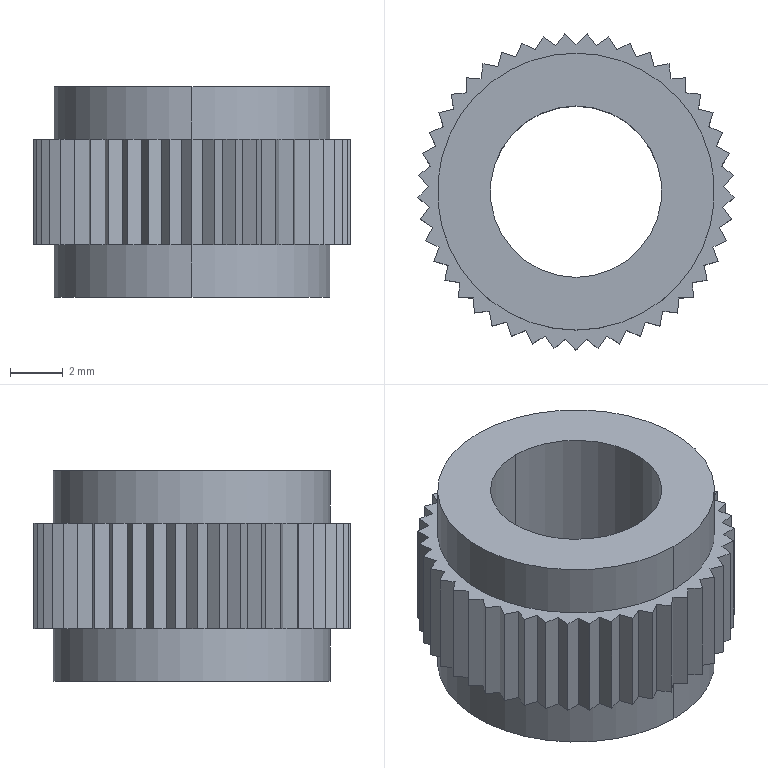Part | SolidWorks | features BaseBody 1 | 1 solid | 100 faces | box 11.993 x 11.985 x 8 mm | volume 502.783 mm3 | plane 94 | cylinder 6 | commonest cylinder face diameters 10.5 x4 6.5 x2